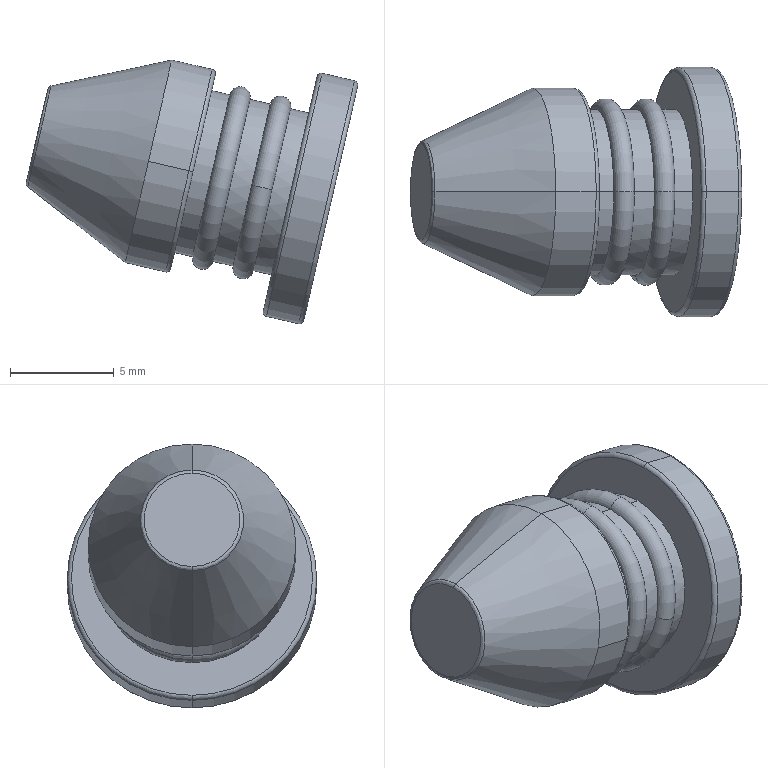Part | SolidWorks | features BaseBody 1 | 1 solid | 37 faces | box 15.957 x 12 x 12.696 mm | volume 692.518 mm3 | torus 15 | cylinder 13 | plane 5 | cone 2 | spline 2 | commonest cylinder face diameters 8 x6 10 x3 5 x2 12 x2
STEP:
#1=CARTESIAN_POINT('',(1987.413,-176.,847.465));
#2=VERTEX_POINT('',#1);
#3=CARTESIAN_POINT('',(1986.898,-173.7,845.223));
#4=VERTEX_POINT('',#3);
#5=CARTESIAN_POINT('',(1986.898,-176.,845.223));
#6=DIRECTION('',(-0.9746,0.,0.2239));
#7=DIRECTION('',(0.2239,0.,0.9746));
#8=AXIS2_PLACEMENT_3D('',#5,#6,#7);
#9=CIRCLE('',#8,2.3);
#10=EDGE_CURVE('',#2,#4,#9,.T.);
#11=ORIENTED_EDGE('',*,*,#10,.T.);
#12=CARTESIAN_POINT('',(1987.093,-173.5,845.178));
#13=VERTEX_POINT('',#12);
#14=CARTESIAN_POINT('',(1987.093,-173.7,845.178));
#15=DIRECTION('',(-0.2239,0.,-0.9746));
#16=DIRECTION('',(-0.9746,0.,0.2239));
#17=AXIS2_PLACEMENT_3D('',#14,#15,#16);
#18=CIRCLE('',#17,0.2);
#19=EDGE_CURVE('',#4,#13,#18,.T.);
#20=ORIENTED_EDGE('',*,*,#19,.T.);
#21=CARTESIAN_POINT('',(1987.652,-176.,847.615));
#22=VERTEX_POINT('',#21);
#23=CARTESIAN_POINT('',(1987.093,-176.,845.178));
#24=DIRECTION('',(-0.9746,0.,0.2239));
#25=DIRECTION('',(0.2239,0.,0.9746));
#26=AXIS2_PLACEMENT_3D('',#23,#24,#25);
#27=CIRCLE('',#26,2.5);
#28=EDGE_CURVE('',#22,#13,#27,.T.);
#29=ORIENTED_EDGE('',*,*,#28,.F.);
#30=CARTESIAN_POINT('',(1987.608,-176.,847.42));
#31=DIRECTION('',(0.,1.,0.));
#32=DIRECTION('',(-0.9746,0.,0.2239));
#33=AXIS2_PLACEMENT_3D('',#30,#31,#32);
#34=CIRCLE('',#33,0.2);
#35=EDGE_CURVE('',#2,#22,#34,.T.);
#36=ORIENTED_EDGE('',*,*,#35,.F.);
#37=EDGE_LOOP('',(#11,#20,#29,#36));
#38=FACE_OUTER_BOUND('',#37,.T.);
#39=CARTESIAN_POINT('',(1987.093,-176.,845.178));
#40=DIRECTION('',(0.9746,0.,-0.2239));
#41=DIRECTION('',(0.,1.,0.));
#42=AXIS2_PLACEMENT_3D('',#39,#40,#41);
#43=TOROIDAL_SURFACE('',#42,2.3,0.2);
#44=ADVANCED_FACE('',(#38),#43,.F.);
#45=CARTESIAN_POINT('',(1993.897,-176.,839.511));
#46=VERTEX_POINT('',#45);
#47=CARTESIAN_POINT('',(1994.792,-180.,843.41));
#48=VERTEX_POINT('',#47);
#49=CARTESIAN_POINT('',(1994.792,-176.,843.41));
#50=DIRECTION('',(-0.9746,0.,0.2239));
#51=DIRECTION('',(-0.2239,0.,-0.9746));
#52=AXIS2_PLACEMENT_3D('',#49,#50,#51);
#53=CIRCLE('',#52,4.);
#54=EDGE_CURVE('',#46,#48,#53,.T.);
#55=ORIENTED_EDGE('',*,*,#54,.T.);
#56=CARTESIAN_POINT('',(1993.818,-180.,843.634));
#57=VERTEX_POINT('',#56);
#58=CARTESIAN_POINT('',(1994.305,-180.,843.522));
#59=DIRECTION('',(-0.2239,0.,-0.9746));
#60=DIRECTION('',(-0.9746,0.,0.2239));
#61=AXIS2_PLACEMENT_3D('',#58,#59,#60);
#62=CIRCLE('',#61,0.5);
#63=EDGE_CURVE('',#48,#57,#62,.T.);
#64=ORIENTED_EDGE('',*,*,#63,.T.);
#65=CARTESIAN_POINT('',(1992.922,-176.,839.735));
#66=VERTEX_POINT('',#65);
#67=CARTESIAN_POINT('',(1993.818,-176.,843.634));
#68=DIRECTION('',(-0.9746,0.,0.2239));
#69=DIRECTION('',(-0.2239,0.,-0.9746));
#70=AXIS2_PLACEMENT_3D('',#67,#68,#69);
#71=CIRCLE('',#70,4.);
#72=EDGE_CURVE('',#66,#57,#71,.T.);
#73=ORIENTED_EDGE('',*,*,#72,.F.);
#74=CARTESIAN_POINT('',(1993.409,-176.,839.623));
#75=DIRECTION('',(0.,1.,0.));
#76=DIRECTION('',(-0.9746,0.,0.2239));
#77=AXIS2_PLACEMENT_3D('',#74,#75,#76);
#78=CIRCLE('',#77,0.5);
#79=EDGE_CURVE('',#46,#66,#78,.T.);
#80=ORIENTED_EDGE('',*,*,#79,.F.);
#81=EDGE_LOOP('',(#55,#64,#73,#80));
#82=FACE_OUTER_BOUND('',#81,.T.);
#83=CARTESIAN_POINT('',(1994.305,-176.,843.522));
#84=DIRECTION('',(-0.9746,0.,0.2239));
#85=DIRECTION('',(0.,-1.,0.));
#86=AXIS2_PLACEMENT_3D('',#83,#84,#85);
#87=TOROIDAL_SURFACE('',#86,4.,0.5);
#88=ADVANCED_FACE('',(#82),#87,.T.);
#89=CARTESIAN_POINT('',(1990.796,-181.,844.328));
#90=VERTEX_POINT('',#89);
#91=CARTESIAN_POINT('',(1989.677,-176.,839.455));
#92=VERTEX_POINT('',#91);
#93=CARTESIAN_POINT('',(1990.796,-176.,844.328));
#94=DIRECTION('',(0.9746,0.,-0.2239));
#95=DIRECTION('',(0.2239,0.,0.9746));
#96=AXIS2_PLACEMENT_3D('',#93,#94,#95);
#97=CIRCLE('',#96,5.);
#98=EDGE_CURVE('',#90,#92,#97,.T.);
#99=ORIENTED_EDGE('',*,*,#98,.F.);
#100=CARTESIAN_POINT('',(1988.847,-181.,844.775));
#101=VERTEX_POINT('',#100);
#102=CARTESIAN_POINT('',(1990.913,-181.,844.301));
#103=DIRECTION('',(-0.9746,0.,0.2239));
#104=VECTOR('',#103,1000.);
#105=LINE('',#102,#104);
#106=EDGE_CURVE('',#90,#101,#105,.T.);
#107=ORIENTED_EDGE('',*,*,#106,.T.);
#108=CARTESIAN_POINT('',(1987.728,-176.,839.902));
#109=VERTEX_POINT('',#108);
#110=CARTESIAN_POINT('',(1988.847,-176.,844.775));
#111=DIRECTION('',(0.9746,0.,-0.2239));
#112=DIRECTION('',(0.2239,0.,0.9746));
#113=AXIS2_PLACEMENT_3D('',#110,#111,#112);
#114=CIRCLE('',#113,5.);
#115=EDGE_CURVE('',#101,#109,#114,.T.);
#116=ORIENTED_EDGE('',*,*,#115,.T.);
#117=CARTESIAN_POINT('',(1987.728,-176.,839.902));
#118=DIRECTION('',(0.9746,0.,-0.2239));
#119=VECTOR('',#118,1000.);
#120=LINE('',#117,#119);
#121=EDGE_CURVE('',#109,#92,#120,.T.);
#122=ORIENTED_EDGE('',*,*,#121,.T.);
#123=EDGE_LOOP('',(#99,#107,#116,#122));
#124=FACE_OUTER_BOUND('',#123,.T.);
#125=CARTESIAN_POINT('',(1990.913,-176.,844.301));
#126=DIRECTION('',(-0.9746,0.,0.2239));
#127=DIRECTION('',(0.,-1.,0.));
#128=AXIS2_PLACEMENT_3D('',#125,#126,#127);
#129=CYLINDRICAL_SURFACE('',#128,5.);
#130=ADVANCED_FACE('',(#124),#129,.T.);
#131=CARTESIAN_POINT('',(1990.991,-180.8,844.283));
#132=VERTEX_POINT('',#131);
#133=CARTESIAN_POINT('',(1989.917,-176.,839.605));
#134=VERTEX_POINT('',#133);
#135=CARTESIAN_POINT('',(1990.991,-176.,844.283));
#136=DIRECTION('',(0.9746,0.,-0.2239));
#137=DIRECTION('',(0.2239,0.,0.9746));
#138=AXIS2_PLACEMENT_3D('',#135,#136,#137);
#139=CIRCLE('',#138,4.8);
#140=EDGE_CURVE('',#132,#134,#139,.T.);
#141=ORIENTED_EDGE('',*,*,#140,.F.);
#142=CARTESIAN_POINT('',(1990.796,-180.8,844.328));
#143=DIRECTION('',(-0.2239,0.,-0.9746));
#144=DIRECTION('',(-0.9746,0.,0.2239));
#145=AXIS2_PLACEMENT_3D('',#142,#143,#144);
#146=CIRCLE('',#145,0.2);
#147=EDGE_CURVE('',#132,#90,#146,.T.);
#148=ORIENTED_EDGE('',*,*,#147,.T.);
#149=ORIENTED_EDGE('',*,*,#98,.T.);
#150=CARTESIAN_POINT('',(1989.722,-176.,839.65));
#151=DIRECTION('',(0.,1.,0.));
#152=DIRECTION('',(-0.2239,0.,-0.9746));
#153=AXIS2_PLACEMENT_3D('',#150,#151,#152);
#154=CIRCLE('',#153,0.2);
#155=EDGE_CURVE('',#134,#92,#154,.T.);
#156=ORIENTED_EDGE('',*,*,#155,.F.);
#157=EDGE_LOOP('',(#141,#148,#149,#156));
#158=FACE_OUTER_BOUND('',#157,.T.);
#159=CARTESIAN_POINT('',(1990.796,-176.,844.328));
#160=DIRECTION('',(-0.9746,0.,0.2239));
#161=DIRECTION('',(0.,-1.,0.));
#162=AXIS2_PLACEMENT_3D('',#159,#160,#161);
#163=TOROIDAL_SURFACE('',#162,4.8,0.2);
#164=ADVANCED_FACE('',(#158),#163,.T.);
#165=CARTESIAN_POINT('',(1990.096,-176.,840.384));
#166=VERTEX_POINT('',#165);
#167=CARTESIAN_POINT('',(1990.973,-176.,840.183));
#168=VERTEX_POINT('',#167);
#169=CARTESIAN_POINT('',(1990.096,-176.,840.384));
#170=DIRECTION('',(0.9746,0.,-0.2239));
#171=VECTOR('',#170,1000.);
#172=LINE('',#169,#171);
#173=EDGE_CURVE('',#166,#168,#172,.T.);
#174=ORIENTED_EDGE('',*,*,#173,.F.);
#175=CARTESIAN_POINT('',(1991.887,-176.,848.181));
#176=VERTEX_POINT('',#175);
#177=CARTESIAN_POINT('',(1990.991,-176.,844.283));
#178=DIRECTION('',(-0.9746,0.,0.2239));
#179=DIRECTION('',(0.2239,0.,0.9746));
#180=AXIS2_PLACEMENT_3D('',#177,#178,#179);
#181=CIRCLE('',#180,4.);
#182=EDGE_CURVE('',#176,#166,#181,.T.);
#183=ORIENTED_EDGE('',*,*,#182,.F.);
#184=CARTESIAN_POINT('',(1992.764,-176.,847.98));
#185=VERTEX_POINT('',#184);
#186=CARTESIAN_POINT('',(1991.887,-176.,848.181));
#187=DIRECTION('',(-0.9746,0.,0.2239));
#188=VECTOR('',#187,1000.);
#189=LINE('',#186,#188);
#190=EDGE_CURVE('',#185,#176,#189,.T.);
#191=ORIENTED_EDGE('',*,*,#190,.F.);
#192=CARTESIAN_POINT('',(1991.868,-176.,844.081));
#193=DIRECTION('',(-0.9746,0.,0.2239));
#194=DIRECTION('',(0.2239,0.,0.9746));
#195=AXIS2_PLACEMENT_3D('',#192,#193,#194);
#196=CIRCLE('',#195,4.);
#197=EDGE_CURVE('',#185,#168,#196,.T.);
#198=ORIENTED_EDGE('',*,*,#197,.T.);
#199=EDGE_LOOP('',(#174,#183,#191,#198));
#200=FACE_OUTER_BOUND('',#199,.T.);
#201=CARTESIAN_POINT('',(1995.786,-176.,843.182));
#202=DIRECTION('',(-0.9746,0.,0.2239));
#203=DIRECTION('',(0.2239,0.,0.9746));
#204=AXIS2_PLACEMENT_3D('',#201,#202,#203);
#205=CYLINDRICAL_SURFACE('',#204,4.);
#206=ADVANCED_FACE('',(#200),#205,.T.);
#207=CARTESIAN_POINT('',(1993.738,-176.,847.756));
#208=VERTEX_POINT('',#207);
#209=CARTESIAN_POINT('',(1994.713,-176.,847.532));
#210=VERTEX_POINT('',#209);
#211=CARTESIAN_POINT('',(1993.738,-176.,847.756));
#212=DIRECTION('',(0.9746,0.,-0.2239));
#213=VECTOR('',#212,1000.);
#214=LINE('',#211,#213);
#215=EDGE_CURVE('',#208,#210,#214,.T.);
#216=ORIENTED_EDGE('',*,*,#215,.T.);
#217=CARTESIAN_POINT('',(1993.818,-176.,843.634));
#218=DIRECTION('',(-0.9746,0.,0.2239));
#219=DIRECTION('',(0.2239,0.,0.9746));
#220=AXIS2_PLACEMENT_3D('',#217,#218,#219);
#221=CIRCLE('',#220,4.);
#222=EDGE_CURVE('',#210,#66,#221,.T.);
#223=ORIENTED_EDGE('',*,*,#222,.T.);
#224=CARTESIAN_POINT('',(1991.948,-176.,839.959));
#225=VERTEX_POINT('',#224);
#226=CARTESIAN_POINT('',(1991.948,-176.,839.959));
#227=DIRECTION('',(-0.9746,0.,0.2239));
#228=VECTOR('',#227,1000.);
#229=LINE('',#226,#228);
#230=EDGE_CURVE('',#66,#225,#229,.T.);
#231=ORIENTED_EDGE('',*,*,#230,.T.);
#232=CARTESIAN_POINT('',(1992.843,-176.,843.858));
#233=DIRECTION('',(-0.9746,0.,0.2239));
#234=DIRECTION('',(0.2239,0.,0.9746));
#235=AXIS2_PLACEMENT_3D('',#232,#233,#234);
#236=CIRCLE('',#235,4.);
#237=EDGE_CURVE('',#208,#225,#236,.T.);
#238=ORIENTED_EDGE('',*,*,#237,.F.);
#239=EDGE_LOOP('',(#216,#223,#231,#238));
#240=FACE_OUTER_BOUND('',#239,.T.);
#241=CARTESIAN_POINT('',(1995.786,-176.,843.182));
#242=DIRECTION('',(-0.9746,0.,0.2239));
#243=DIRECTION('',(0.2239,0.,0.9746));
#244=AXIS2_PLACEMENT_3D('',#241,#242,#243);
#245=CYLINDRICAL_SURFACE('',#244,4.);
#246=ADVANCED_FACE('',(#240),#245,.T.);
#247=CARTESIAN_POINT('',(1996.565,-176.,847.107));
#248=VERTEX_POINT('',#247);
#249=CARTESIAN_POINT('',(1995.688,-176.,847.308));
#250=VERTEX_POINT('',#249);
#251=CARTESIAN_POINT('',(1995.688,-176.,847.308));
#252=DIRECTION('',(-0.9746,0.,0.2239));
#253=VECTOR('',#252,1000.);
#254=LINE('',#251,#253);
#255=EDGE_CURVE('',#248,#250,#254,.T.);
#256=ORIENTED_EDGE('',*,*,#255,.F.);
#257=CARTESIAN_POINT('',(1994.774,-176.,839.31));
#258=VERTEX_POINT('',#257);
#259=CARTESIAN_POINT('',(1995.669,-176.,843.208));
#260=DIRECTION('',(-0.9746,0.,0.2239));
#261=DIRECTION('',(0.2239,0.,0.9746));
#262=AXIS2_PLACEMENT_3D('',#259,#260,#261);
#263=CIRCLE('',#262,4.);
#264=EDGE_CURVE('',#248,#258,#263,.T.);
#265=ORIENTED_EDGE('',*,*,#264,.T.);
#266=CARTESIAN_POINT('',(1993.897,-176.,839.511));
#267=DIRECTION('',(0.9746,0.,-0.2239));
#268=VECTOR('',#267,1000.);
#269=LINE('',#266,#268);
#270=EDGE_CURVE('',#46,#258,#269,.T.);
#271=ORIENTED_EDGE('',*,*,#270,.F.);
#272=CARTESIAN_POINT('',(1994.792,-176.,843.41));
#273=DIRECTION('',(-0.9746,0.,0.2239));
#274=DIRECTION('',(0.2239,0.,0.9746));
#275=AXIS2_PLACEMENT_3D('',#272,#273,#274);
#276=CIRCLE('',#275,4.);
#277=EDGE_CURVE('',#250,#46,#276,.T.);
#278=ORIENTED_EDGE('',*,*,#277,.F.);
#279=EDGE_LOOP('',(#256,#265,#271,#278));
#280=FACE_OUTER_BOUND('',#279,.T.);
#281=CARTESIAN_POINT('',(1995.786,-176.,843.182));
#282=DIRECTION('',(-0.9746,0.,0.2239));
#283=DIRECTION('',(0.2239,0.,0.9746));
#284=AXIS2_PLACEMENT_3D('',#281,#282,#283);
#285=CYLINDRICAL_SURFACE('',#284,4.);
#286=ADVANCED_FACE('',(#280),#285,.T.);
#287=CARTESIAN_POINT('',(1993.251,-176.,847.868));
#288=DIRECTION('',(0.,1.,0.));
#289=DIRECTION('',(-0.9746,0.,0.2239));
#290=AXIS2_PLACEMENT_3D('',#287,#288,#289);
#291=CIRCLE('',#290,0.5);
#292=EDGE_CURVE('',#185,#208,#291,.T.);
#293=ORIENTED_EDGE('',*,*,#292,.T.);
#294=ORIENTED_EDGE('',*,*,#237,.T.);
#295=CARTESIAN_POINT('',(1991.46,-176.,840.071));
#296=DIRECTION('',(0.,1.,0.));
#297=DIRECTION('',(-0.9746,0.,0.2239));
#298=AXIS2_PLACEMENT_3D('',#295,#296,#297);
#299=CIRCLE('',#298,0.5);
#300=EDGE_CURVE('',#225,#168,#299,.T.);
#301=ORIENTED_EDGE('',*,*,#300,.T.);
#302=ORIENTED_EDGE('',*,*,#197,.F.);
#303=EDGE_LOOP('',(#293,#294,#301,#302));
#304=FACE_OUTER_BOUND('',#303,.T.);
#305=CARTESIAN_POINT('',(1992.356,-176.,843.97));
#306=DIRECTION('',(-0.9746,0.,0.2239));
#307=DIRECTION('',(0.2239,0.,0.9746));
#308=AXIS2_PLACEMENT_3D('',#305,#306,#307);
#309=TOROIDAL_SURFACE('',#308,4.,0.5);
#310=ADVANCED_FACE('',(#304),#309,.T.);
#311=ORIENTED_EDGE('',*,*,#300,.F.);
#312=CARTESIAN_POINT('',(1992.843,-176.,843.858));
#313=DIRECTION('',(-0.9746,0.,0.2239));
#314=DIRECTION('',(-0.2239,0.,-0.9746));
#315=AXIS2_PLACEMENT_3D('',#312,#313,#314);
#316=CIRCLE('',#315,4.);
#317=EDGE_CURVE('',#225,#208,#316,.T.);
#318=ORIENTED_EDGE('',*,*,#317,.T.);
#319=ORIENTED_EDGE('',*,*,#292,.F.);
#320=CARTESIAN_POINT('',(1991.868,-176.,844.081));
#321=DIRECTION('',(-0.9746,0.,0.2239));
#322=DIRECTION('',(-0.2239,0.,-0.9746));
#323=AXIS2_PLACEMENT_3D('',#320,#321,#322);
#324=CIRCLE('',#323,4.);
#325=EDGE_CURVE('',#168,#185,#324,.T.);
#326=ORIENTED_EDGE('',*,*,#325,.F.);
#327=EDGE_LOOP('',(#311,#318,#319,#326));
#328=FACE_OUTER_BOUND('',#327,.T.);
#329=CARTESIAN_POINT('',(1992.356,-176.,843.97));
#330=DIRECTION('',(-0.9746,0.,0.2239));
#331=DIRECTION('',(0.2239,0.,0.9746));
#332=AXIS2_PLACEMENT_3D('',#329,#330,#331);
#333=TOROIDAL_SURFACE('',#332,4.,0.5);
#334=ADVANCED_FACE('',(#328),#333,.T.);
#335=ORIENTED_EDGE('',*,*,#190,.T.);
#336=CARTESIAN_POINT('',(1990.991,-176.,844.283));
#337=DIRECTION('',(-0.9746,0.,0.2239));
#338=DIRECTION('',(-0.2239,0.,-0.9746));
#339=AXIS2_PLACEMENT_3D('',#336,#337,#338);
#340=CIRCLE('',#339,4.);
#341=EDGE_CURVE('',#166,#176,#340,.T.);
#342=ORIENTED_EDGE('',*,*,#341,.F.);
#343=ORIENTED_EDGE('',*,*,#173,.T.);
#344=ORIENTED_EDGE('',*,*,#325,.T.);
#345=EDGE_LOOP('',(#335,#342,#343,#344));
#346=FACE_OUTER_BOUND('',#345,.T.);
#347=CARTESIAN_POINT('',(1995.786,-176.,843.182));
#348=DIRECTION('',(-0.9746,0.,0.2239));
#349=DIRECTION('',(0.2239,0.,0.9746));
#350=AXIS2_PLACEMENT_3D('',#347,#348,#349);
#351=CYLINDRICAL_SURFACE('',#350,4.);
#352=ADVANCED_FACE('',(#346),#351,.T.);
#353=ORIENTED_EDGE('',*,*,#230,.F.);
#354=ORIENTED_EDGE('',*,*,#72,.T.);
#355=CARTESIAN_POINT('',(1993.818,-176.,843.634));
#356=DIRECTION('',(-0.9746,0.,0.2239));
#357=DIRECTION('',(-0.2239,0.,-0.9746));
#358=AXIS2_PLACEMENT_3D('',#355,#356,#357);
#359=CIRCLE('',#358,4.);
#360=EDGE_CURVE('',#57,#210,#359,.T.);
#361=ORIENTED_EDGE('',*,*,#360,.T.);
#362=ORIENTED_EDGE('',*,*,#215,.F.);
#363=ORIENTED_EDGE('',*,*,#317,.F.);
#364=EDGE_LOOP('',(#353,#354,#361,#362,#363));
#365=FACE_OUTER_BOUND('',#364,.T.);
#366=CARTESIAN_POINT('',(1995.786,-176.,843.182));
#367=DIRECTION('',(-0.9746,0.,0.2239));
#368=DIRECTION('',(0.2239,0.,0.9746));
#369=AXIS2_PLACEMENT_3D('',#366,#367,#368);
#370=CYLINDRICAL_SURFACE('',#369,4.);
#371=ADVANCED_FACE('',(#365),#370,.T.);
#372=ORIENTED_EDGE('',*,*,#270,.T.);
#373=CARTESIAN_POINT('',(1995.669,-176.,843.208));
#374=DIRECTION('',(0.9746,0.,-0.2239));
#375=DIRECTION('',(0.2239,0.,0.9746));
#376=AXIS2_PLACEMENT_3D('',#373,#374,#375);
#377=CIRCLE('',#376,4.);
#378=EDGE_CURVE('',#248,#258,#377,.T.);
#379=ORIENTED_EDGE('',*,*,#378,.F.);
#380=ORIENTED_EDGE('',*,*,#255,.T.);
#381=CARTESIAN_POINT('',(1994.792,-176.,843.41));
#382=DIRECTION('',(-0.9746,0.,0.2239));
#383=DIRECTION('',(-0.2239,0.,-0.9746));
#384=AXIS2_PLACEMENT_3D('',#381,#382,#383);
#385=CIRCLE('',#384,4.);
#386=EDGE_CURVE('',#48,#250,#385,.T.);
#387=ORIENTED_EDGE('',*,*,#386,.F.);
#388=ORIENTED_EDGE('',*,*,#54,.F.);
#389=EDGE_LOOP('',(#372,#379,#380,#387,#388));
#390=FACE_OUTER_BOUND('',#389,.T.);
#391=CARTESIAN_POINT('',(1995.786,-176.,843.182));
#392=DIRECTION('',(-0.9746,0.,0.2239));
#393=DIRECTION('',(0.2239,0.,0.9746));
#394=AXIS2_PLACEMENT_3D('',#391,#392,#393);
#395=CYLINDRICAL_SURFACE('',#394,4.);
#396=ADVANCED_FACE('',(#390),#395,.T.);
#397=CARTESIAN_POINT('',(1992.066,-176.,848.961));
#398=VERTEX_POINT('',#397);
#399=CARTESIAN_POINT('',(1990.991,-176.,844.283));
#400=DIRECTION('',(-0.9746,0.,0.2239));
#401=DIRECTION('',(0.2239,0.,0.9746));
#402=AXIS2_PLACEMENT_3D('',#399,#400,#401);
#403=CIRCLE('',#402,4.8);
#404=EDGE_CURVE('',#398,#134,#403,.T.);
#405=ORIENTED_EDGE('',*,*,#404,.F.);
#406=CARTESIAN_POINT('',(1990.991,-176.,844.283));
#407=DIRECTION('',(0.9746,0.,-0.2239));
#408=DIRECTION('',(0.2239,0.,0.9746));
#409=AXIS2_PLACEMENT_3D('',#406,#407,#408);
#410=CIRCLE('',#409,4.8);
#411=EDGE_CURVE('',#398,#132,#410,.T.);
#412=ORIENTED_EDGE('',*,*,#411,.T.);
#413=ORIENTED_EDGE('',*,*,#140,.T.);
#414=EDGE_LOOP('',(#405,#412,#413));
#415=FACE_OUTER_BOUND('',#414,.T.);
#416=ORIENTED_EDGE('',*,*,#341,.T.);
#417=ORIENTED_EDGE('',*,*,#182,.T.);
#418=EDGE_LOOP('',(#416,#417));
#419=FACE_BOUND('',#418,.T.);
#420=CARTESIAN_POINT('',(1992.109,-170.987,849.148));
#421=DIRECTION('',(0.9746,0.,-0.2239));
#422=DIRECTION('',(0.,-1.,0.));
#423=AXIS2_PLACEMENT_3D('',#420,#421,#422);
#424=PLANE('',#423);
#425=ADVANCED_FACE('',(#415,#419),#424,.T.);
#426=ORIENTED_EDGE('',*,*,#147,.F.);
#427=ORIENTED_EDGE('',*,*,#411,.F.);
#428=CARTESIAN_POINT('',(1991.916,-176.,849.201));
#429=VERTEX_POINT('',#428);
#430=CARTESIAN_POINT('',(1991.871,-176.,849.006));
#431=DIRECTION('',(0.,1.,0.));
#432=DIRECTION('',(0.2239,0.,0.9746));
#433=AXIS2_PLACEMENT_3D('',#430,#431,#432);
#434=CIRCLE('',#433,0.2);
#435=EDGE_CURVE('',#429,#398,#434,.T.);
#436=ORIENTED_EDGE('',*,*,#435,.F.);
#437=CARTESIAN_POINT('',(1990.796,-176.,844.328));
#438=DIRECTION('',(0.9746,0.,-0.2239));
#439=DIRECTION('',(0.2239,0.,0.9746));
#440=AXIS2_PLACEMENT_3D('',#437,#438,#439);
#441=CIRCLE('',#440,5.);
#442=EDGE_CURVE('',#429,#90,#441,.T.);
#443=ORIENTED_EDGE('',*,*,#442,.T.);
#444=EDGE_LOOP('',(#426,#427,#436,#443));
#445=FACE_OUTER_BOUND('',#444,.T.);
#446=CARTESIAN_POINT('',(1990.796,-176.,844.328));
#447=DIRECTION('',(-0.9746,0.,0.2239));
#448=DIRECTION('',(0.,-1.,0.));
#449=AXIS2_PLACEMENT_3D('',#446,#447,#448);
#450=TOROIDAL_SURFACE('',#449,4.8,0.2);
#451=ADVANCED_FACE('',(#445),#450,.T.);
#452=ORIENTED_EDGE('',*,*,#404,.T.);
#453=ORIENTED_EDGE('',*,*,#155,.T.);
#454=CARTESIAN_POINT('',(1990.796,-176.,844.328));
#455=DIRECTION('',(-0.9746,0.,0.2239));
#456=DIRECTION('',(0.2239,0.,0.9746));
#457=AXIS2_PLACEMENT_3D('',#454,#455,#456);
#458=CIRCLE('',#457,5.);
#459=EDGE_CURVE('',#429,#92,#458,.T.);
#460=ORIENTED_EDGE('',*,*,#459,.F.);
#461=ORIENTED_EDGE('',*,*,#435,.T.);
#462=EDGE_LOOP('',(#452,#453,#460,#461));
#463=FACE_OUTER_BOUND('',#462,.T.);
#464=CARTESIAN_POINT('',(1990.796,-176.,844.328));
#465=DIRECTION('',(-0.9746,0.,0.2239));
#466=DIRECTION('',(0.,-1.,0.));
#467=AXIS2_PLACEMENT_3D('',#464,#465,#466);
#468=TOROIDAL_SURFACE('',#467,4.8,0.2);
#469=ADVANCED_FACE('',(#463),#468,.T.);
#470=ORIENTED_EDGE('',*,*,#459,.T.);
#471=ORIENTED_EDGE('',*,*,#121,.F.);
#472=CARTESIAN_POINT('',(1989.966,-176.,849.649));
#473=VERTEX_POINT('',#472);
#474=CARTESIAN_POINT('',(1988.847,-176.,844.775));
#475=DIRECTION('',(-0.9746,0.,0.2239));
#476=DIRECTION('',(0.2239,0.,0.9746));
#477=AXIS2_PLACEMENT_3D('',#474,#475,#476);
#478=CIRCLE('',#477,5.);
#479=EDGE_CURVE('',#473,#109,#478,.T.);
#480=ORIENTED_EDGE('',*,*,#479,.F.);
#481=CARTESIAN_POINT('',(1989.966,-176.,849.649));
#482=DIRECTION('',(-0.9746,0.,0.2239));
#483=VECTOR('',#482,1000.);
#484=LINE('',#481,#483);
#485=EDGE_CURVE('',#429,#473,#484,.T.);
#486=ORIENTED_EDGE('',*,*,#485,.F.);
#487=EDGE_LOOP('',(#470,#471,#480,#486));
#488=FACE_OUTER_BOUND('',#487,.T.);
#489=CARTESIAN_POINT('',(1990.913,-176.,844.301));
#490=DIRECTION('',(-0.9746,0.,0.2239));
#491=DIRECTION('',(0.,-1.,0.));
#492=AXIS2_PLACEMENT_3D('',#489,#490,#491);
#493=CYLINDRICAL_SURFACE('',#492,5.);
#494=ADVANCED_FACE('',(#488),#493,.T.);
#495=ORIENTED_EDGE('',*,*,#106,.F.);
#496=ORIENTED_EDGE('',*,*,#442,.F.);
#497=ORIENTED_EDGE('',*,*,#485,.T.);
#498=CARTESIAN_POINT('',(1988.847,-176.,844.775));
#499=DIRECTION('',(0.9746,0.,-0.2239));
#500=DIRECTION('',(0.2239,0.,0.9746));
#501=AXIS2_PLACEMENT_3D('',#498,#499,#500);
#502=CIRCLE('',#501,5.);
#503=EDGE_CURVE('',#473,#101,#502,.T.);
#504=ORIENTED_EDGE('',*,*,#503,.T.);
#505=EDGE_LOOP('',(#495,#496,#497,#504));
#506=FACE_OUTER_BOUND('',#505,.T.);
#507=CARTESIAN_POINT('',(1990.913,-176.,844.301));
#508=DIRECTION('',(-0.9746,0.,0.2239));
#509=DIRECTION('',(0.,-1.,0.));
#510=AXIS2_PLACEMENT_3D('',#507,#508,#509);
#511=CYLINDRICAL_SURFACE('',#510,5.);
#512=ADVANCED_FACE('',(#506),#511,.T.);
#513=CARTESIAN_POINT('',(1984.156,-176.,848.407));
#514=VERTEX_POINT('',#513);
#515=CARTESIAN_POINT('',(1983.042,-176.,843.555));
#516=VERTEX_POINT('',#515);
#517=CARTESIAN_POINT('',(1983.599,-176.,845.981));
#518=DIRECTION('',(0.9746,0.,-0.2239));
#519=DIRECTION('',(0.2239,0.,0.9746));
#520=AXIS2_PLACEMENT_3D('',#517,#518,#519);
#521=CIRCLE('',#520,2.489);
#522=EDGE_CURVE('',#514,#516,#521,.T.);
#523=ORIENTED_EDGE('',*,*,#522,.T.);
#524=CARTESIAN_POINT('',(1983.042,-176.,843.555));
#525=DIRECTION('',(-0.7887,0.,0.6148));
#526=VECTOR('',#525,1000.);
#527=LINE('',#524,#526);
#528=EDGE_CURVE('',#109,#516,#527,.T.);
#529=ORIENTED_EDGE('',*,*,#528,.F.);
#530=ORIENTED_EDGE('',*,*,#115,.F.);
#531=ORIENTED_EDGE('',*,*,#503,.F.);
#532=CARTESIAN_POINT('',(1984.156,-176.,848.407));
#533=DIRECTION('',(0.9779,0.,0.209));
#534=VECTOR('',#533,1000.);
#535=LINE('',#532,#534);
#536=EDGE_CURVE('',#514,#473,#535,.T.);
#537=ORIENTED_EDGE('',*,*,#536,.F.);
#538=EDGE_LOOP('',(#523,#529,#530,#531,#537));
#539=FACE_OUTER_BOUND('',#538,.T.);
#540=CARTESIAN_POINT('',(1988.953,-176.,844.751));
#541=DIRECTION('',(0.9746,0.,-0.2239));
#542=DIRECTION('',(-0.2239,0.,-0.9746));
#543=AXIS2_PLACEMENT_3D('',#540,#541,#542);
#544=CONICAL_SURFACE('',#543,5.051,0.4363);
#545=ADVANCED_FACE('',(#539),#544,.T.);
#546=ORIENTED_EDGE('',*,*,#479,.T.);
#547=ORIENTED_EDGE('',*,*,#528,.T.);
#548=CARTESIAN_POINT('',(1983.599,-176.,845.981));
#549=DIRECTION('',(-0.9746,0.,0.2239));
#550=DIRECTION('',(0.2239,0.,0.9746));
#551=AXIS2_PLACEMENT_3D('',#548,#549,#550);
#552=CIRCLE('',#551,2.489);
#553=EDGE_CURVE('',#514,#516,#552,.T.);
#554=ORIENTED_EDGE('',*,*,#553,.F.);
#555=ORIENTED_EDGE('',*,*,#536,.T.);
#556=EDGE_LOOP('',(#546,#547,#554,#555));
#557=FACE_OUTER_BOUND('',#556,.T.);
#558=CARTESIAN_POINT('',(1988.953,-176.,844.751));
#559=DIRECTION('',(0.9746,0.,-0.2239));
#560=DIRECTION('',(-0.2239,0.,-0.9746));
#561=AXIS2_PLACEMENT_3D('',#558,#559,#560);
#562=CONICAL_SURFACE('',#561,5.051,0.4363);
#563=ADVANCED_FACE('',(#557),#562,.T.);
#564=ORIENTED_EDGE('',*,*,#553,.T.);
#565=CARTESIAN_POINT('',(1982.97,-176.,843.757));
#566=VERTEX_POINT('',#565);
#567=CARTESIAN_POINT('',(1983.165,-176.,843.713));
#568=DIRECTION('',(0.,-1.,0.));
#569=DIRECTION('',(-0.9746,0.,0.2239));
#570=AXIS2_PLACEMENT_3D('',#567,#568,#569);
#571=CIRCLE('',#570,0.2);
#572=EDGE_CURVE('',#566,#516,#571,.T.);
#573=ORIENTED_EDGE('',*,*,#572,.F.);
#574=CARTESIAN_POINT('',(1984.003,-176.,848.256));
#575=VERTEX_POINT('',#574);
#576=CARTESIAN_POINT('',(1983.487,-176.,846.007));
#577=DIRECTION('',(-0.9746,0.,0.2239));
#578=DIRECTION('',(0.2239,0.,0.9746));
#579=AXIS2_PLACEMENT_3D('',#576,#577,#578);
#580=CIRCLE('',#579,2.308);
#581=EDGE_CURVE('',#575,#566,#580,.T.);
#582=ORIENTED_EDGE('',*,*,#581,.F.);
#583=CARTESIAN_POINT('',(1984.198,-176.,848.211));
#584=DIRECTION('',(0.,-1.,0.));
#585=DIRECTION('',(-0.9746,0.,0.2239));
#586=AXIS2_PLACEMENT_3D('',#583,#584,#585);
#587=CIRCLE('',#586,0.2);
#588=EDGE_CURVE('',#514,#575,#587,.T.);
#589=ORIENTED_EDGE('',*,*,#588,.F.);
#590=EDGE_LOOP('',(#564,#573,#582,#589));
#591=FACE_OUTER_BOUND('',#590,.T.);
#592=CARTESIAN_POINT('',(1984.16,-176.156,848.403));
#593=CARTESIAN_POINT('',(1984.078,-176.154,848.387));
#594=CARTESIAN_POINT('',(1984.018,-176.15,848.329));
#595=CARTESIAN_POINT('',(1984.001,-176.145,848.247));
#596=CARTESIAN_POINT('',(1984.181,-174.626,848.497));
#597=CARTESIAN_POINT('',(1984.099,-174.645,848.48));
#598=CARTESIAN_POINT('',(1984.039,-174.684,848.419));
#599=CARTESIAN_POINT('',(1984.021,-174.73,848.334));
#600=CARTESIAN_POINT('',(1983.946,-173.509,847.474));
#601=CARTESIAN_POINT('',(1983.867,-173.543,847.471));
#602=CARTESIAN_POINT('',(1983.814,-173.613,847.439));
#603=CARTESIAN_POINT('',(1983.804,-173.697,847.388));
#604=CARTESIAN_POINT('',(1983.603,-173.509,845.98));
#605=CARTESIAN_POINT('',(1983.529,-173.543,845.997));
#606=CARTESIAN_POINT('',(1983.485,-173.613,846.007));
#607=CARTESIAN_POINT('',(1983.487,-173.697,846.007));
#608=CARTESIAN_POINT('',(1983.26,-173.509,844.486));
#609=CARTESIAN_POINT('',(1983.19,-173.543,844.523));
#610=CARTESIAN_POINT('',(1983.156,-173.613,844.575));
#611=CARTESIAN_POINT('',(1983.169,-173.697,844.625));
#612=CARTESIAN_POINT('',(1983.025,-174.626,843.463));
#613=CARTESIAN_POINT('',(1982.958,-174.645,843.514));
#614=CARTESIAN_POINT('',(1982.931,-174.684,843.595));
#615=CARTESIAN_POINT('',(1982.952,-174.73,843.679));
#616=CARTESIAN_POINT('',(1983.047,-176.156,843.557));
#617=CARTESIAN_POINT('',(1982.98,-176.154,843.607));
#618=CARTESIAN_POINT('',(1982.952,-176.15,843.685));
#619=CARTESIAN_POINT('',(1982.972,-176.145,843.766));
#620=(BOUNDED_SURFACE()B_SPLINE_SURFACE(3,3,((#592,#593,#594,#595),(#596,#597,#598,#599),(#600,#601,#602,#603),(#604,#605,#606,#607),(#608,#609,#610,#611),(#612,#613,#614,#615),(#616,#617,#618,#619)),.UNSPECIFIED.,.F.,.F.,.T.)B_SPLINE_SURFACE_WITH_KNOTS((4,3,4),(4,4),(0.,0.5,1.),(0.,1.),.UNSPECIFIED.)GEOMETRIC_REPRESENTATION_ITEM()RATIONAL_B_SPLINE_SURFACE(((1.297,1.151,1.151,1.297),(1.024,0.9087,0.9087,1.024),(1.024,0.9087,0.9087,1.024),(1.297,1.151,1.151,1.297),(1.024,0.9087,0.9087,1.024),(1.024,0.9087,0.9087,1.024),(1.297,1.151,1.151,1.297)))REPRESENTATION_ITEM('')SURFACE());
#621=ADVANCED_FACE('',(#591),#620,.T.);
#622=CARTESIAN_POINT('',(1983.487,-176.,846.007));
#623=DIRECTION('',(0.9746,0.,-0.2239));
#624=DIRECTION('',(0.2239,0.,0.9746));
#625=AXIS2_PLACEMENT_3D('',#622,#623,#624);
#626=CIRCLE('',#625,2.308);
#627=EDGE_CURVE('',#575,#566,#626,.T.);
#628=ORIENTED_EDGE('',*,*,#627,.T.);
#629=ORIENTED_EDGE('',*,*,#572,.T.);
#630=ORIENTED_EDGE('',*,*,#522,.F.);
#631=ORIENTED_EDGE('',*,*,#588,.T.);
#632=EDGE_LOOP('',(#628,#629,#630,#631));
#633=FACE_OUTER_BOUND('',#632,.T.);
#634=CARTESIAN_POINT('',(1983.047,-175.844,843.557));
#635=CARTESIAN_POINT('',(1982.98,-175.846,843.607));
#636=CARTESIAN_POINT('',(1982.952,-175.85,843.685));
#637=CARTESIAN_POINT('',(1982.972,-175.855,843.766));
#638=CARTESIAN_POINT('',(1983.025,-177.374,843.463));
#639=CARTESIAN_POINT('',(1982.958,-177.355,843.514));
#640=CARTESIAN_POINT('',(1982.931,-177.316,843.595));
#641=CARTESIAN_POINT('',(1982.952,-177.27,843.679));
#642=CARTESIAN_POINT('',(1983.26,-178.491,844.486));
#643=CARTESIAN_POINT('',(1983.19,-178.457,844.523));
#644=CARTESIAN_POINT('',(1983.156,-178.387,844.575));
#645=CARTESIAN_POINT('',(1983.169,-178.303,844.625));
#646=CARTESIAN_POINT('',(1983.603,-178.491,845.98));
#647=CARTESIAN_POINT('',(1983.529,-178.457,845.997));
#648=CARTESIAN_POINT('',(1983.485,-178.387,846.007));
#649=CARTESIAN_POINT('',(1983.487,-178.303,846.007));
#650=CARTESIAN_POINT('',(1983.946,-178.491,847.474));
#651=CARTESIAN_POINT('',(1983.867,-178.457,847.471));
#652=CARTESIAN_POINT('',(1983.814,-178.387,847.439));
#653=CARTESIAN_POINT('',(1983.804,-178.303,847.388));
#654=CARTESIAN_POINT('',(1984.181,-177.374,848.497));
#655=CARTESIAN_POINT('',(1984.099,-177.355,848.48));
#656=CARTESIAN_POINT('',(1984.039,-177.316,848.419));
#657=CARTESIAN_POINT('',(1984.021,-177.27,848.334));
#658=CARTESIAN_POINT('',(1984.16,-175.844,848.403));
#659=CARTESIAN_POINT('',(1984.078,-175.846,848.387));
#660=CARTESIAN_POINT('',(1984.018,-175.85,848.329));
#661=CARTESIAN_POINT('',(1984.001,-175.855,848.247));
#662=(BOUNDED_SURFACE()B_SPLINE_SURFACE(3,3,((#634,#635,#636,#637),(#638,#639,#640,#641),(#642,#643,#644,#645),(#646,#647,#648,#649),(#650,#651,#652,#653),(#654,#655,#656,#657),(#658,#659,#660,#661)),.UNSPECIFIED.,.F.,.F.,.F.)B_SPLINE_SURFACE_WITH_KNOTS((4,3,4),(4,4),(0.,0.5,1.),(0.,1.),.UNSPECIFIED.)GEOMETRIC_REPRESENTATION_ITEM()RATIONAL_B_SPLINE_SURFACE(((1.297,1.151,1.151,1.297),(1.024,0.9087,0.9087,1.024),(1.024,0.9087,0.9087,1.024),(1.297,1.151,1.151,1.297),(1.024,0.9087,0.9087,1.024),(1.024,0.9087,0.9087,1.024),(1.297,1.151,1.151,1.297)))REPRESENTATION_ITEM('')SURFACE());
#663=ADVANCED_FACE('',(#633),#662,.T.);
#664=ORIENTED_EDGE('',*,*,#581,.T.);
#665=ORIENTED_EDGE('',*,*,#627,.F.);
#666=EDGE_LOOP('',(#664,#665));
#667=FACE_OUTER_BOUND('',#666,.T.);
#668=CARTESIAN_POINT('',(1984.03,-173.558,848.373));
#669=DIRECTION('',(-0.9746,0.,0.2239));
#670=DIRECTION('',(-0.2239,0.,-0.9746));
#671=AXIS2_PLACEMENT_3D('',#668,#669,#670);
#672=PLANE('',#671);
#673=ADVANCED_FACE('',(#667),#672,.T.);
#674=ORIENTED_EDGE('',*,*,#63,.F.);
#675=ORIENTED_EDGE('',*,*,#386,.T.);
#676=CARTESIAN_POINT('',(1995.2,-176.,847.42));
#677=DIRECTION('',(0.,1.,0.));
#678=DIRECTION('',(-0.9746,0.,0.2239));
#679=AXIS2_PLACEMENT_3D('',#676,#677,#678);
#680=CIRCLE('',#679,0.5);
#681=EDGE_CURVE('',#210,#250,#680,.T.);
#682=ORIENTED_EDGE('',*,*,#681,.F.);
#683=ORIENTED_EDGE('',*,*,#360,.F.);
#684=EDGE_LOOP('',(#674,#675,#682,#683));
#685=FACE_OUTER_BOUND('',#684,.T.);
#686=CARTESIAN_POINT('',(1994.305,-176.,843.522));
#687=DIRECTION('',(-0.9746,0.,0.2239));
#688=DIRECTION('',(0.,-1.,0.));
#689=AXIS2_PLACEMENT_3D('',#686,#687,#688);
#690=TOROIDAL_SURFACE('',#689,4.,0.5);
#691=ADVANCED_FACE('',(#685),#690,.T.);
#692=ORIENTED_EDGE('',*,*,#681,.T.);
#693=ORIENTED_EDGE('',*,*,#277,.T.);
#694=ORIENTED_EDGE('',*,*,#79,.T.);
#695=ORIENTED_EDGE('',*,*,#222,.F.);
#696=EDGE_LOOP('',(#692,#693,#694,#695));
#697=FACE_OUTER_BOUND('',#696,.T.);
#698=CARTESIAN_POINT('',(1994.305,-176.,843.522));
#699=DIRECTION('',(-0.9746,0.,0.2239));
#700=DIRECTION('',(0.,-1.,0.));
#701=AXIS2_PLACEMENT_3D('',#698,#699,#700);
#702=TOROIDAL_SURFACE('',#701,4.,0.5);
#703=ADVANCED_FACE('',(#697),#702,.T.);
#704=CARTESIAN_POINT('',(1996.968,-176.,848.861));
#705=VERTEX_POINT('',#704);
#706=CARTESIAN_POINT('',(1994.371,-176.,837.556));
#707=VERTEX_POINT('',#706);
#708=CARTESIAN_POINT('',(1995.669,-176.,843.208));
#709=DIRECTION('',(-0.9746,0.,0.2239));
#710=DIRECTION('',(0.2239,0.,0.9746));
#711=AXIS2_PLACEMENT_3D('',#708,#709,#710);
#712=CIRCLE('',#711,5.8);
#713=EDGE_CURVE('',#705,#707,#712,.T.);
#714=ORIENTED_EDGE('',*,*,#713,.T.);
#715=CARTESIAN_POINT('',(1995.669,-176.,843.208));
#716=DIRECTION('',(0.9746,0.,-0.2239));
#717=DIRECTION('',(0.2239,0.,0.9746));
#718=AXIS2_PLACEMENT_3D('',#715,#716,#717);
#719=CIRCLE('',#718,5.8);
#720=EDGE_CURVE('',#705,#707,#719,.T.);
#721=ORIENTED_EDGE('',*,*,#720,.F.);
#722=EDGE_LOOP('',(#714,#721));
#723=FACE_OUTER_BOUND('',#722,.T.);
#724=ORIENTED_EDGE('',*,*,#378,.T.);
#725=ORIENTED_EDGE('',*,*,#264,.F.);
#726=EDGE_LOOP('',(#724,#725));
#727=FACE_BOUND('',#726,.T.);
#728=CARTESIAN_POINT('',(1997.02,-169.968,849.087));
#729=DIRECTION('',(-0.9746,0.,0.2239));
#730=DIRECTION('',(-0.2239,0.,-0.9746));
#731=AXIS2_PLACEMENT_3D('',#728,#729,#730);
#732=PLANE('',#731);
#733=ADVANCED_FACE('',(#723,#727),#732,.T.);
#734=ORIENTED_EDGE('',*,*,#720,.T.);
#735=CARTESIAN_POINT('',(1994.521,-176.,837.316));
#736=VERTEX_POINT('',#735);
#737=CARTESIAN_POINT('',(1994.566,-176.,837.511));
#738=DIRECTION('',(0.,-1.,0.));
#739=DIRECTION('',(-0.9746,0.,0.2239));
#740=AXIS2_PLACEMENT_3D('',#737,#738,#739);
#741=CIRCLE('',#740,0.2);
#742=EDGE_CURVE('',#707,#736,#741,.T.);
#743=ORIENTED_EDGE('',*,*,#742,.T.);
#744=CARTESIAN_POINT('',(1997.208,-176.,849.011));
#745=VERTEX_POINT('',#744);
#746=CARTESIAN_POINT('',(1995.864,-176.,843.164));
#747=DIRECTION('',(0.9746,0.,-0.2239));
#748=DIRECTION('',(0.2239,0.,0.9746));
#749=AXIS2_PLACEMENT_3D('',#746,#747,#748);
#750=CIRCLE('',#749,6.);
#751=EDGE_CURVE('',#745,#736,#750,.T.);
#752=ORIENTED_EDGE('',*,*,#751,.F.);
#753=CARTESIAN_POINT('',(1997.163,-176.,848.816));
#754=DIRECTION('',(0.,-1.,0.));
#755=DIRECTION('',(-0.9746,0.,0.2239));
#756=AXIS2_PLACEMENT_3D('',#753,#754,#755);
#757=CIRCLE('',#756,0.2);
#758=EDGE_CURVE('',#745,#705,#757,.T.);
#759=ORIENTED_EDGE('',*,*,#758,.T.);
#760=EDGE_LOOP('',(#734,#743,#752,#759));
#761=FACE_OUTER_BOUND('',#760,.T.);
#762=CARTESIAN_POINT('',(1995.864,-176.,843.164));
#763=DIRECTION('',(-0.9746,0.,0.2239));
#764=DIRECTION('',(0.2239,0.,0.9746));
#765=AXIS2_PLACEMENT_3D('',#762,#763,#764);
#766=TOROIDAL_SURFACE('',#765,5.8,0.2);
#767=ADVANCED_FACE('',(#761),#766,.T.);
#768=CARTESIAN_POINT('',(1995.864,-176.,843.164));
#769=DIRECTION('',(-0.9746,0.,0.2239));
#770=DIRECTION('',(0.2239,0.,0.9746));
#771=AXIS2_PLACEMENT_3D('',#768,#769,#770);
#772=CIRCLE('',#771,6.);
#773=EDGE_CURVE('',#745,#736,#772,.T.);
#774=ORIENTED_EDGE('',*,*,#773,.T.);
#775=ORIENTED_EDGE('',*,*,#742,.F.);
#776=ORIENTED_EDGE('',*,*,#713,.F.);
#777=ORIENTED_EDGE('',*,*,#758,.F.);
#778=EDGE_LOOP('',(#774,#775,#776,#777));
#779=FACE_OUTER_BOUND('',#778,.T.);
#780=CARTESIAN_POINT('',(1995.864,-176.,843.164));
#781=DIRECTION('',(-0.9746,0.,0.2239));
#782=DIRECTION('',(0.2239,0.,0.9746));
#783=AXIS2_PLACEMENT_3D('',#780,#781,#782);
#784=TOROIDAL_SURFACE('',#783,5.8,0.2);
#785=ADVANCED_FACE('',(#779),#784,.T.);
#786=CARTESIAN_POINT('',(1998.767,-176.,848.653));
#787=VERTEX_POINT('',#786);
#788=CARTESIAN_POINT('',(1996.081,-176.,836.958));
#789=VERTEX_POINT('',#788);
#790=CARTESIAN_POINT('',(1997.424,-176.,842.805));
#791=DIRECTION('',(-0.9746,0.,0.2239));
#792=DIRECTION('',(0.2239,0.,0.9746));
#793=AXIS2_PLACEMENT_3D('',#790,#791,#792);
#794=CIRCLE('',#793,6.);
#795=EDGE_CURVE('',#787,#789,#794,.T.);
#796=ORIENTED_EDGE('',*,*,#795,.T.);
#797=CARTESIAN_POINT('',(1994.521,-176.,837.316));
#798=DIRECTION('',(0.9746,0.,-0.2239));
#799=VECTOR('',#798,1000.);
#800=LINE('',#797,#799);
#801=EDGE_CURVE('',#736,#789,#800,.T.);
#802=ORIENTED_EDGE('',*,*,#801,.F.);
#803=ORIENTED_EDGE('',*,*,#773,.F.);
#804=CARTESIAN_POINT('',(1997.208,-176.,849.011));
#805=DIRECTION('',(-0.9746,0.,0.2239));
#806=VECTOR('',#805,1000.);
#807=LINE('',#804,#806);
#808=EDGE_CURVE('',#787,#745,#807,.T.);
#809=ORIENTED_EDGE('',*,*,#808,.F.);
#810=EDGE_LOOP('',(#796,#802,#803,#809));
#811=FACE_OUTER_BOUND('',#810,.T.);
#812=CARTESIAN_POINT('',(1997.541,-176.,842.779));
#813=DIRECTION('',(-0.9746,0.,0.2239));
#814=DIRECTION('',(0.2239,0.,0.9746));
#815=AXIS2_PLACEMENT_3D('',#812,#813,#814);
#816=CYLINDRICAL_SURFACE('',#815,6.);
#817=ADVANCED_FACE('',(#811),#816,.T.);
#818=ORIENTED_EDGE('',*,*,#751,.T.);
#819=ORIENTED_EDGE('',*,*,#801,.T.);
#820=CARTESIAN_POINT('',(1997.424,-176.,842.805));
#821=DIRECTION('',(0.9746,0.,-0.2239));
#822=DIRECTION('',(0.2239,0.,0.9746));
#823=AXIS2_PLACEMENT_3D('',#820,#821,#822);
#824=CIRCLE('',#823,6.);
#825=EDGE_CURVE('',#787,#789,#824,.T.);
#826=ORIENTED_EDGE('',*,*,#825,.F.);
#827=ORIENTED_EDGE('',*,*,#808,.T.);
#828=EDGE_LOOP('',(#818,#819,#826,#827));
#829=FACE_OUTER_BOUND('',#828,.T.);
#830=CARTESIAN_POINT('',(1997.541,-176.,842.779));
#831=DIRECTION('',(-0.9746,0.,0.2239));
#832=DIRECTION('',(0.2239,0.,0.9746));
#833=AXIS2_PLACEMENT_3D('',#830,#831,#832);
#834=CYLINDRICAL_SURFACE('',#833,6.);
#835=ADVANCED_FACE('',(#829),#834,.T.);
#836=ORIENTED_EDGE('',*,*,#825,.T.);
#837=CARTESIAN_POINT('',(1996.32,-176.,837.108));
#838=VERTEX_POINT('',#837);
#839=CARTESIAN_POINT('',(1996.125,-176.,837.153));
#840=DIRECTION('',(0.,-1.,0.));
#841=DIRECTION('',(-0.2239,0.,-0.9746));
#842=AXIS2_PLACEMENT_3D('',#839,#840,#841);
#843=CIRCLE('',#842,0.2);
#844=EDGE_CURVE('',#789,#838,#843,.T.);
#845=ORIENTED_EDGE('',*,*,#844,.T.);
#846=CARTESIAN_POINT('',(1998.917,-176.,848.413));
#847=VERTEX_POINT('',#846);
#848=CARTESIAN_POINT('',(1997.619,-176.,842.761));
#849=DIRECTION('',(0.9746,0.,-0.2239));
#850=DIRECTION('',(0.2239,0.,0.9746));
#851=AXIS2_PLACEMENT_3D('',#848,#849,#850);
#852=CIRCLE('',#851,5.8);
#853=EDGE_CURVE('',#847,#838,#852,.T.);
#854=ORIENTED_EDGE('',*,*,#853,.F.);
#855=CARTESIAN_POINT('',(1998.722,-176.,848.458));
#856=DIRECTION('',(0.,-1.,0.));
#857=DIRECTION('',(0.2239,0.,0.9746));
#858=AXIS2_PLACEMENT_3D('',#855,#856,#857);
#859=CIRCLE('',#858,0.2);
#860=EDGE_CURVE('',#847,#787,#859,.T.);
#861=ORIENTED_EDGE('',*,*,#860,.T.);
#862=EDGE_LOOP('',(#836,#845,#854,#861));
#863=FACE_OUTER_BOUND('',#862,.T.);
#864=CARTESIAN_POINT('',(1997.424,-176.,842.805));
#865=DIRECTION('',(-0.9746,0.,0.2239));
#866=DIRECTION('',(0.2239,0.,0.9746));
#867=AXIS2_PLACEMENT_3D('',#864,#865,#866);
#868=TOROIDAL_SURFACE('',#867,5.8,0.2);
#869=ADVANCED_FACE('',(#863),#868,.T.);
#870=CARTESIAN_POINT('',(1997.619,-176.,842.761));
#871=DIRECTION('',(-0.9746,0.,0.2239));
#872=DIRECTION('',(0.2239,0.,0.9746));
#873=AXIS2_PLACEMENT_3D('',#870,#871,#872);
#874=CIRCLE('',#873,5.8);
#875=EDGE_CURVE('',#847,#838,#874,.T.);
#876=ORIENTED_EDGE('',*,*,#875,.T.);
#877=ORIENTED_EDGE('',*,*,#844,.F.);
#878=ORIENTED_EDGE('',*,*,#795,.F.);
#879=ORIENTED_EDGE('',*,*,#860,.F.);
#880=EDGE_LOOP('',(#876,#877,#878,#879));
#881=FACE_OUTER_BOUND('',#880,.T.);
#882=CARTESIAN_POINT('',(1997.424,-176.,842.805));
#883=DIRECTION('',(-0.9746,0.,0.2239));
#884=DIRECTION('',(0.2239,0.,0.9746));
#885=AXIS2_PLACEMENT_3D('',#882,#883,#884);
#886=TOROIDAL_SURFACE('',#885,5.8,0.2);
#887=ADVANCED_FACE('',(#881),#886,.T.);
#888=ORIENTED_EDGE('',*,*,#875,.F.);
#889=ORIENTED_EDGE('',*,*,#853,.T.);
#890=EDGE_LOOP('',(#888,#889));
#891=FACE_OUTER_BOUND('',#890,.T.);
#892=CARTESIAN_POINT('',(1997.059,-176.,840.324));
#893=VERTEX_POINT('',#892);
#894=CARTESIAN_POINT('',(1998.178,-176.,845.197));
#895=VERTEX_POINT('',#894);
#896=CARTESIAN_POINT('',(1997.619,-176.,842.761));
#897=DIRECTION('',(0.9746,0.,-0.2239));
#898=DIRECTION('',(-0.2239,0.,-0.9746));
#899=AXIS2_PLACEMENT_3D('',#896,#897,#898);
#900=CIRCLE('',#899,2.5);
#901=EDGE_CURVE('',#893,#895,#900,.T.);
#902=ORIENTED_EDGE('',*,*,#901,.F.);
#903=CARTESIAN_POINT('',(1997.619,-176.,842.761));
#904=DIRECTION('',(0.9746,0.,-0.2239));
#905=DIRECTION('',(0.2239,0.,0.9746));
#906=AXIS2_PLACEMENT_3D('',#903,#904,#905);
#907=CIRCLE('',#906,2.5);
#908=EDGE_CURVE('',#895,#893,#907,.T.);
#909=ORIENTED_EDGE('',*,*,#908,.F.);
#910=EDGE_LOOP('',(#902,#909));
#911=FACE_BOUND('',#910,.T.);
#912=CARTESIAN_POINT('',(1998.969,-169.968,848.64));
#913=DIRECTION('',(0.9746,0.,-0.2239));
#914=DIRECTION('',(0.,-1.,0.));
#915=AXIS2_PLACEMENT_3D('',#912,#913,#914);
#916=PLANE('',#915);
#917=ADVANCED_FACE('',(#891,#911),#916,.T.);
#918=ORIENTED_EDGE('',*,*,#908,.T.);
#919=CARTESIAN_POINT('',(1986.533,-176.,842.742));
#920=VERTEX_POINT('',#919);
#921=CARTESIAN_POINT('',(1986.533,-176.,842.742));
#922=DIRECTION('',(0.9746,0.,-0.2239));
#923=VECTOR('',#922,1000.);
#924=LINE('',#921,#923);
#925=EDGE_CURVE('',#920,#893,#924,.T.);
#926=ORIENTED_EDGE('',*,*,#925,.F.);
#927=CARTESIAN_POINT('',(1987.093,-176.,845.178));
#928=DIRECTION('',(0.9746,0.,-0.2239));
#929=DIRECTION('',(0.2239,0.,0.9746));
#930=AXIS2_PLACEMENT_3D('',#927,#928,#929);
#931=CIRCLE('',#930,2.5);
#932=EDGE_CURVE('',#22,#920,#931,.T.);
#933=ORIENTED_EDGE('',*,*,#932,.F.);
#934=CARTESIAN_POINT('',(1987.652,-176.,847.615));
#935=DIRECTION('',(-0.9746,0.,0.2239));
#936=VECTOR('',#935,1000.);
#937=LINE('',#934,#936);
#938=EDGE_CURVE('',#895,#22,#937,.T.);
#939=ORIENTED_EDGE('',*,*,#938,.F.);
#940=EDGE_LOOP('',(#918,#926,#933,#939));
#941=FACE_OUTER_BOUND('',#940,.T.);
#942=CARTESIAN_POINT('',(1986.882,-176.,845.227));
#943=DIRECTION('',(0.9746,0.,-0.2239));
#944=DIRECTION('',(-0.2239,0.,-0.9746));
#945=AXIS2_PLACEMENT_3D('',#942,#943,#944);
#946=CYLINDRICAL_SURFACE('',#945,2.5);
#947=ADVANCED_FACE('',(#941),#946,.F.);
#948=ORIENTED_EDGE('',*,*,#28,.T.);
#949=CARTESIAN_POINT('',(1987.093,-176.,845.178));
#950=DIRECTION('',(-0.9746,0.,0.2239));
#951=DIRECTION('',(0.2239,0.,0.9746));
#952=AXIS2_PLACEMENT_3D('',#949,#950,#951);
#953=CIRCLE('',#952,2.5);
#954=EDGE_CURVE('',#13,#920,#953,.T.);
#955=ORIENTED_EDGE('',*,*,#954,.T.);
#956=ORIENTED_EDGE('',*,*,#925,.T.);
#957=ORIENTED_EDGE('',*,*,#901,.T.);
#958=ORIENTED_EDGE('',*,*,#938,.T.);
#959=EDGE_LOOP('',(#948,#955,#956,#957,#958));
#960=FACE_OUTER_BOUND('',#959,.T.);
#961=CARTESIAN_POINT('',(1986.882,-176.,845.227));
#962=DIRECTION('',(0.9746,0.,-0.2239));
#963=DIRECTION('',(-0.2239,0.,-0.9746));
#964=AXIS2_PLACEMENT_3D('',#961,#962,#963);
#965=CYLINDRICAL_SURFACE('',#964,2.5);
#966=ADVANCED_FACE('',(#960),#965,.F.);
#967=ORIENTED_EDGE('',*,*,#19,.F.);
#968=CARTESIAN_POINT('',(1986.383,-176.,842.982));
#969=VERTEX_POINT('',#968);
#970=CARTESIAN_POINT('',(1986.898,-176.,845.223));
#971=DIRECTION('',(-0.9746,0.,0.2239));
#972=DIRECTION('',(0.2239,0.,0.9746));
#973=AXIS2_PLACEMENT_3D('',#970,#971,#972);
#974=CIRCLE('',#973,2.3);
#975=EDGE_CURVE('',#4,#969,#974,.T.);
#976=ORIENTED_EDGE('',*,*,#975,.T.);
#977=CARTESIAN_POINT('',(1986.578,-176.,842.937));
#978=DIRECTION('',(0.,1.,0.));
#979=DIRECTION('',(-0.9746,0.,0.2239));
#980=AXIS2_PLACEMENT_3D('',#977,#978,#979);
#981=CIRCLE('',#980,0.2);
#982=EDGE_CURVE('',#920,#969,#981,.T.);
#983=ORIENTED_EDGE('',*,*,#982,.F.);
#984=ORIENTED_EDGE('',*,*,#954,.F.);
#985=EDGE_LOOP('',(#967,#976,#983,#984));
#986=FACE_OUTER_BOUND('',#985,.T.);
#987=CARTESIAN_POINT('',(1987.093,-176.,845.178));
#988=DIRECTION('',(0.9746,0.,-0.2239));
#989=DIRECTION('',(0.,1.,0.));
#990=AXIS2_PLACEMENT_3D('',#987,#988,#989);
#991=TOROIDAL_SURFACE('',#990,2.3,0.2);
#992=ADVANCED_FACE('',(#986),#991,.F.);
#993=ORIENTED_EDGE('',*,*,#932,.T.);
#994=ORIENTED_EDGE('',*,*,#982,.T.);
#995=CARTESIAN_POINT('',(1986.898,-176.,845.223));
#996=DIRECTION('',(0.9746,0.,-0.2239));
#997=DIRECTION('',(0.2239,0.,0.9746));
#998=AXIS2_PLACEMENT_3D('',#995,#996,#997);
#999=CIRCLE('',#998,2.3);
#1000=EDGE_CURVE('',#2,#969,#999,.T.);
#1001=ORIENTED_EDGE('',*,*,#1000,.F.);
#1002=ORIENTED_EDGE('',*,*,#35,.T.);
#1003=EDGE_LOOP('',(#993,#994,#1001,#1002));
#1004=FACE_OUTER_BOUND('',#1003,.T.);
#1005=CARTESIAN_POINT('',(1987.093,-176.,845.178));
#1006=DIRECTION('',(0.9746,0.,-0.2239));
#1007=DIRECTION('',(0.,1.,0.));
#1008=AXIS2_PLACEMENT_3D('',#1005,#1006,#1007);
#1009=TOROIDAL_SURFACE('',#1008,2.3,0.2);
#1010=ADVANCED_FACE('',(#1004),#1009,.F.);
#1011=ORIENTED_EDGE('',*,*,#1000,.T.);
#1012=ORIENTED_EDGE('',*,*,#975,.F.);
#1013=ORIENTED_EDGE('',*,*,#10,.F.);
#1014=EDGE_LOOP('',(#1011,#1012,#1013));
#1015=FACE_OUTER_BOUND('',#1014,.T.);
#1016=CARTESIAN_POINT('',(1986.356,-173.565,842.865));
#1017=DIRECTION('',(0.9746,0.,-0.2239));
#1018=DIRECTION('',(0.2239,0.,0.9746));
#1019=AXIS2_PLACEMENT_3D('',#1016,#1017,#1018);
#1020=PLANE('',#1019);
#1021=ADVANCED_FACE('',(#1015),#1020,.T.);
#1022=CLOSED_SHELL('',(#44,#88,#130,#164,#206,#246,#286,#310,#334,#352,#371,#396,#425,#451,#469,#494,#512,#545,#563,#621,#663,#673,#691,#703,#733,#767,#785,#817,#835,#869,#887,#917,#947,#966,#992,#1010,#1021));
#1023=MANIFOLD_SOLID_BREP('',#1022);
#1024=CARTESIAN_POINT('',(0.,0.,0.));
#1025=DIRECTION('',(0.,0.,1.));
#1026=DIRECTION('',(1.,0.,0.));
#1027=AXIS2_PLACEMENT_3D('',#1024,#1025,#1026);
#1028=(LENGTH_UNIT()NAMED_UNIT(*)SI_UNIT(.MILLI.,.METRE.));
#1029=UNCERTAINTY_MEASURE_WITH_UNIT(LENGTH_MEASURE(0.00001),#1028,'','');
#1030=(NAMED_UNIT(*)PLANE_ANGLE_UNIT()SI_UNIT($,.RADIAN.));
#1031=(NAMED_UNIT(*)SI_UNIT($,.STERADIAN.)SOLID_ANGLE_UNIT());
#1032=(GEOMETRIC_REPRESENTATION_CONTEXT(3)GLOBAL_UNCERTAINTY_ASSIGNED_CONTEXT((#1029))GLOBAL_UNIT_ASSIGNED_CONTEXT((#1028,#1030,#1031))REPRESENTATION_CONTEXT('',''));
#1033=ADVANCED_BREP_SHAPE_REPRESENTATION('',(#1023,#1027),#1032);